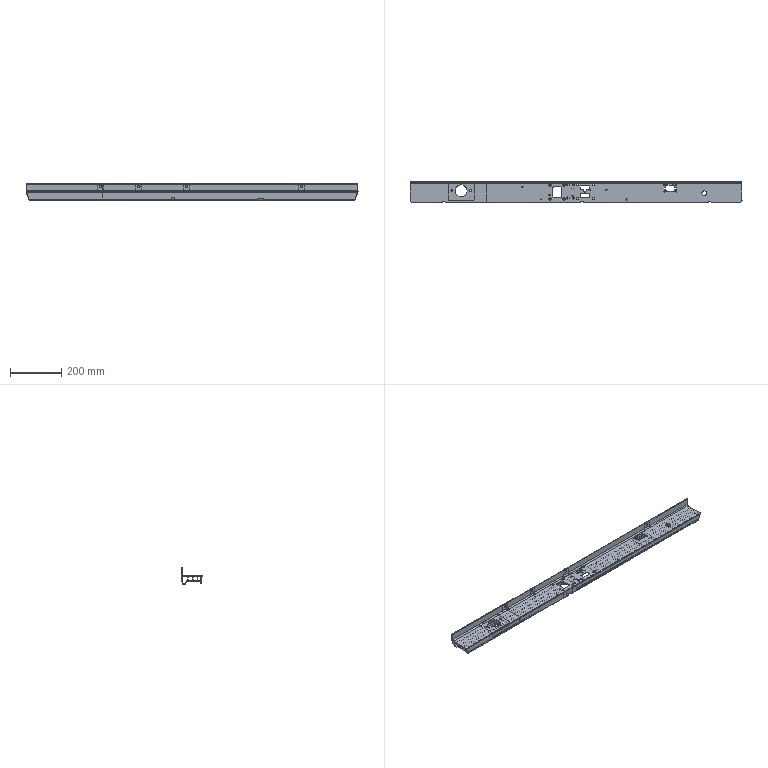NC program | NX | posted with a generic post | part box 1301 x 81.1 x 63 mm
Lines 11162 to 11296 of 19512:
(HOLE_MILLING_1 , TOOL : D6)
N22262 T06 M6
N22264 G54
N22266 G17 G0 G90 X-101.6 Y27.134 B0. C0. S6000 M3
N22268 G43 Z30. H6
N22270 Z-29.5
N22272 G94 G3 X-100.912 Y26.447 R0.688 F1400.
N22274 X-100.225 Y27.134 R0.688
N22276 X-100.225 Y27.134 Z-30. I-1.375 J0.
N22278 X-100.225 Y27.134 Z-30.5 I-1.375 J0.
N22280 X-100.225 Y27.134 Z-31. I-1.375 J0.
N22282 X-100.225 Y27.134 Z-31.5 I-1.375 J0.
N22284 X-100.225 Y27.134 Z-32. I-1.375 J0.
N22286 X-100.225 Y27.134 Z-32.5 I-1.375 J0.
N22288 X-100.225 Y27.134 Z-33. I-1.375 J0.
N22290 X-101.6 Y28.509 R1.375
N22292 X-100.225 Y27.134 R-1.375
N22294 X-100.912 Y27.822 R0.688
N22296 X-101.6 Y27.134 R0.688
N22298 G0 Z30.
N22300 Y-27.366
N22302 Z-29.5
N22304 G3 X-100.912 Y-28.054 R0.688
N22306 X-100.225 Y-27.366 R0.688
N22308 X-100.225 Y-27.366 Z-30. I-1.375 J0.
N22310 X-100.225 Y-27.366 Z-30.5 I-1.375 J0.
N22312 X-100.225 Y-27.366 Z-31. I-1.375 J0.
N22314 X-100.225 Y-27.366 Z-31.5 I-1.375 J0.
N22316 X-100.225 Y-27.366 Z-32. I-1.375 J0.
N22318 X-100.225 Y-27.366 Z-32.5 I-1.375 J0.
N22320 X-100.225 Y-27.366 Z-33. I-1.375 J0.
N22322 X-101.6 Y-25.991 R1.375
N22324 X-100.225 Y-27.366 R-1.375
N22326 X-100.912 Y-26.679 R0.688
N22328 X-101.6 Y-27.366 R0.688
N22330 G0 Z30.
N22332 X-47.1 Y27.134
N22334 Z-29.5
N22336 G3 X-46.412 Y26.447 R0.688
N22338 X-45.725 Y27.134 R0.688
N22340 X-45.725 Y27.134 Z-30. I-1.375 J0.
N22342 X-45.725 Y27.134 Z-30.5 I-1.375 J0.
N22344 X-45.725 Y27.134 Z-31. I-1.375 J0.
N22346 X-45.725 Y27.134 Z-31.5 I-1.375 J0.
N22348 X-45.725 Y27.134 Z-32. I-1.375 J0.
N22350 X-45.725 Y27.134 Z-32.5 I-1.375 J0.
N22352 X-45.725 Y27.134 Z-33. I-1.375 J0.
N22354 X-47.1 Y28.509 R1.375
N22356 X-45.725 Y27.134 R-1.375
N22358 X-46.412 Y27.822 R0.688
N22360 X-47.1 Y27.134 R0.688
N22362 G0 Z30.
N22364 Y-27.366
N22366 Z-29.5
N22368 G3 X-46.412 Y-28.054 R0.688
N22370 X-45.725 Y-27.366 R0.688
N22372 X-45.725 Y-27.366 Z-30. I-1.375 J0.
N22374 X-45.725 Y-27.366 Z-30.5 I-1.375 J0.
N22376 X-45.725 Y-27.366 Z-31. I-1.375 J0.
N22378 X-45.725 Y-27.366 Z-31.5 I-1.375 J0.
N22380 X-45.725 Y-27.366 Z-32. I-1.375 J0.
N22382 X-45.725 Y-27.366 Z-32.5 I-1.375 J0.
N22384 X-45.725 Y-27.366 Z-33. I-1.375 J0.
N22386 X-47.1 Y-25.991 R1.375
N22388 X-45.725 Y-27.366 R-1.375
N22390 X-46.412 Y-26.679 R0.688
N22392 X-47.1 Y-27.366 R0.688
N22394 G0 Z30.
N22396 X4.8 Y29.646
N22398 Z-29.5
N22400 G3 X5.487 Y28.958 R0.688
N22402 X6.175 Y29.646 R0.688
N22404 X6.175 Y29.646 Z-30. I-1.375 J0.
N22406 X6.175 Y29.646 Z-30.5 I-1.375 J0.
N22408 X6.175 Y29.646 Z-31. I-1.375 J0.
N22410 X6.175 Y29.646 Z-31.5 I-1.375 J0.
N22412 X6.175 Y29.646 Z-32. I-1.375 J0.
N22414 X6.175 Y29.646 Z-32.5 I-1.375 J0.
N22416 X6.175 Y29.646 Z-33. I-1.375 J0.
N22418 X4.8 Y31.021 R1.375
N22420 X6.175 Y29.646 R-1.375
N22422 X5.487 Y30.333 R0.688
N22424 X4.8 Y29.646 R0.688
N22426 G0 Z30.
N22428 Y-25.354
N22430 Z-29.5
N22432 G3 X5.487 Y-26.042 R0.688
N22434 X6.175 Y-25.354 R0.688
N22436 X6.175 Y-25.354 Z-30. I-1.375 J0.
N22438 X6.175 Y-25.354 Z-30.5 I-1.375 J0.
N22440 X6.175 Y-25.354 Z-31. I-1.375 J0.
N22442 X6.175 Y-25.354 Z-31.5 I-1.375 J0.
N22444 X6.175 Y-25.354 Z-32. I-1.375 J0.
N22446 X6.175 Y-25.354 Z-32.5 I-1.375 J0.
N22448 X6.175 Y-25.354 Z-33. I-1.375 J0.
N22450 X4.8 Y-23.979 R1.375
N22452 X6.175 Y-25.354 R-1.375
N22454 X5.487 Y-24.667 R0.688
N22456 X4.8 Y-25.354 R0.688
N22458 G0 Z30.
N22460 X68.8 Y29.646
N22462 Z-29.5
N22464 G3 X69.487 Y28.958 R0.688
N22466 X70.175 Y29.646 R0.688
N22468 X70.175 Y29.646 Z-30. I-1.375 J0.
N22470 X70.175 Y29.646 Z-30.5 I-1.375 J0.
N22472 X70.175 Y29.646 Z-31. I-1.375 J0.
N22474 X70.175 Y29.646 Z-31.5 I-1.375 J0.
N22476 X70.175 Y29.646 Z-32. I-1.375 J0.
N22478 X70.175 Y29.646 Z-32.5 I-1.375 J0.
N22480 X70.175 Y29.646 Z-33. I-1.375 J0.
N22482 X68.8 Y31.021 R1.375
N22484 X70.175 Y29.646 R-1.375
N22486 X69.487 Y30.333 R0.688
N22488 X68.8 Y29.646 R0.688
N22490 G0 Z30.
N22492 Y-25.354
N22494 Z-29.5
N22496 G3 X69.487 Y-26.042 R0.688
N22498 X70.175 Y-25.354 R0.688
N22500 X70.175 Y-25.354 Z-30. I-1.375 J0.
N22502 X70.175 Y-25.354 Z-30.5 I-1.375 J0.
N22504 X70.175 Y-25.354 Z-31. I-1.375 J0.
N22506 X70.175 Y-25.354 Z-31.5 I-1.375 J0.
N22508 X70.175 Y-25.354 Z-32. I-1.375 J0.
N22510 X70.175 Y-25.354 Z-32.5 I-1.375 J0.
N22512 X70.175 Y-25.354 Z-33. I-1.375 J0.
N22514 X68.8 Y-23.979 R1.375
N22516 X70.175 Y-25.354 R-1.375
N22518 X69.487 Y-24.667 R0.688
N22520 X68.8 Y-25.354 R0.688
N22522 G0 Z30.
N22524 M5